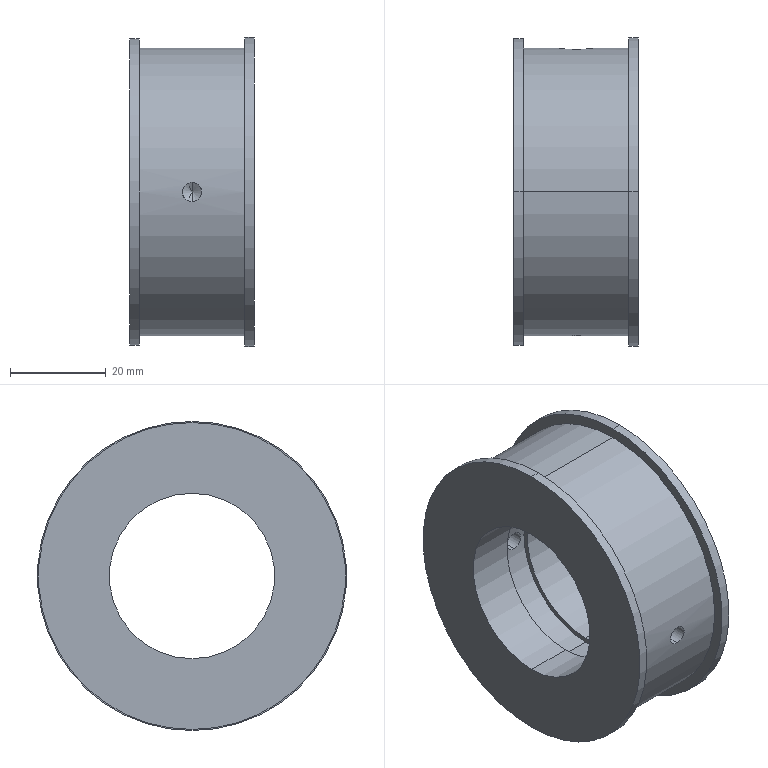Part | SolidWorks | features HoleWzd 3, Fillet 2, Revolution 1 | 1 solid | 31 faces | box 26 x 64.446 x 64.446 mm | volume 49939 mm3 | cylinder 18 | plane 7 | torus 2 | spline 2 | cone 2 | commonest cylinder face diameters 4 x4 34.5 x4 7.5 x2 36.5 x2 60 x2 64 x2
STEP:
#1=CARTESIAN_POINT('',(4.61,28.8,3.75));
#2=VERTEX_POINT('',#1);
#3=CARTESIAN_POINT('',(4.61,28.8,-3.75));
#4=VERTEX_POINT('',#3);
#5=CARTESIAN_POINT('',(4.61,28.8,0.));
#6=DIRECTION('',(0.,-1.,0.));
#7=DIRECTION('',(0.,0.,-1.));
#8=AXIS2_PLACEMENT_3D('',#5,#6,#7);
#9=CIRCLE('',#8,3.75);
#10=EDGE_CURVE('',#2,#4,#9,.T.);
#11=ORIENTED_EDGE('',*,*,#10,.F.);
#12=CARTESIAN_POINT('',(4.61,28.5,3.45));
#13=VERTEX_POINT('',#12);
#14=CARTESIAN_POINT('',(4.61,28.8,3.45));
#15=DIRECTION('',(1.,0.,0.));
#16=DIRECTION('',(0.,0.,-1.));
#17=AXIS2_PLACEMENT_3D('',#14,#15,#16);
#18=CIRCLE('',#17,0.3);
#19=EDGE_CURVE('',#2,#13,#18,.T.);
#20=ORIENTED_EDGE('',*,*,#19,.T.);
#21=CARTESIAN_POINT('',(4.61,28.5,-3.45));
#22=VERTEX_POINT('',#21);
#23=CARTESIAN_POINT('',(4.61,28.5,0.));
#24=DIRECTION('',(0.,1.,0.));
#25=DIRECTION('',(0.,0.,-1.));
#26=AXIS2_PLACEMENT_3D('',#23,#24,#25);
#27=CIRCLE('',#26,3.45);
#28=EDGE_CURVE('',#22,#13,#27,.T.);
#29=ORIENTED_EDGE('',*,*,#28,.F.);
#30=CARTESIAN_POINT('',(4.61,28.8,-3.45));
#31=DIRECTION('',(-1.,0.,0.));
#32=DIRECTION('',(0.,0.,1.));
#33=AXIS2_PLACEMENT_3D('',#30,#31,#32);
#34=CIRCLE('',#33,0.3);
#35=EDGE_CURVE('',#4,#22,#34,.T.);
#36=ORIENTED_EDGE('',*,*,#35,.F.);
#37=EDGE_LOOP('',(#11,#20,#29,#36));
#38=FACE_OUTER_BOUND('',#37,.T.);
#39=CARTESIAN_POINT('',(4.61,28.8,0.));
#40=DIRECTION('',(0.,-1.,0.));
#41=DIRECTION('',(0.,0.,-1.));
#42=AXIS2_PLACEMENT_3D('',#39,#40,#41);
#43=TOROIDAL_SURFACE('',#42,3.45,0.3);
#44=ADVANCED_FACE('',(#38),#43,.F.);
#45=CARTESIAN_POINT('',(3.758,29.551,-3.652));
#46=VERTEX_POINT('',#45);
#47=CARTESIAN_POINT('',(4.61,29.537,3.75));
#48=VERTEX_POINT('',#47);
#49=CARTESIAN_POINT('',(3.758,29.551,-3.652));
#50=CARTESIAN_POINT('',(3.535,29.558,-3.6));
#51=CARTESIAN_POINT('',(3.316,29.568,-3.527));
#52=CARTESIAN_POINT('',(2.899,29.591,-3.345));
#53=CARTESIAN_POINT('',(2.701,29.605,-3.236));
#54=CARTESIAN_POINT('',(2.325,29.634,-2.982));
#55=CARTESIAN_POINT('',(2.146,29.65,-2.836));
#56=CARTESIAN_POINT('',(1.822,29.682,-2.518));
#57=CARTESIAN_POINT('',(1.676,29.698,-2.346));
#58=CARTESIAN_POINT('',(1.414,29.728,-1.974));
#59=CARTESIAN_POINT('',(1.299,29.742,-1.774));
#60=CARTESIAN_POINT('',(1.109,29.766,-1.363));
#61=CARTESIAN_POINT('',(1.033,29.776,-1.149));
#62=CARTESIAN_POINT('',(0.9203,29.792,-0.7059));
#63=CARTESIAN_POINT('',(0.8842,29.797,-0.479));
#64=CARTESIAN_POINT('',(0.8536,29.801,-0.02683));
#65=CARTESIAN_POINT('',(0.8587,29.8,0.2003));
#66=CARTESIAN_POINT('',(0.9112,29.793,0.6567));
#67=CARTESIAN_POINT('',(0.9579,29.786,0.8794));
#68=CARTESIAN_POINT('',(1.09,29.769,1.312));
#69=CARTESIAN_POINT('',(1.177,29.757,1.524));
#70=CARTESIAN_POINT('',(1.387,29.731,1.93));
#71=CARTESIAN_POINT('',(1.509,29.717,2.121));
#72=CARTESIAN_POINT('',(1.787,29.686,2.478));
#73=CARTESIAN_POINT('',(1.944,29.67,2.647));
#74=CARTESIAN_POINT('',(2.284,29.638,2.95));
#75=CARTESIAN_POINT('',(2.466,29.623,3.084));
#76=CARTESIAN_POINT('',(2.853,29.594,3.32));
#77=CARTESIAN_POINT('',(3.06,29.581,3.422));
#78=CARTESIAN_POINT('',(3.485,29.56,3.584));
#79=CARTESIAN_POINT('',(3.703,29.552,3.646));
#80=CARTESIAN_POINT('',(4.15,29.54,3.729));
#81=CARTESIAN_POINT('',(4.38,29.537,3.75));
#82=CARTESIAN_POINT('',(4.61,29.537,3.75));
#83=B_SPLINE_CURVE_WITH_KNOTS('',3,(#49,#50,#51,#52,#53,#54,#55,#56,#57,#58,#59,#60,#61,#62,#63,#64,#65,#66,#67,#68,#69,#70,#71,#72,#73,#74,#75,#76,#77,#78,#79,#80,#81,#82),.UNSPECIFIED.,.F.,.F.,(4,2,2,2,2,2,2,2,2,2,2,2,2,2,2,2,4),(0.01269,0.01337,0.01406,0.01474,0.01543,0.01611,0.0168,0.01748,0.01817,0.01885,0.01954,0.02022,0.02091,0.02159,0.02228,0.02296,0.02365),.UNSPECIFIED.);
#84=EDGE_CURVE('',#46,#48,#83,.T.);
#85=ORIENTED_EDGE('',*,*,#84,.F.);
#86=CARTESIAN_POINT('',(3.712,29.749,-3.872));
#87=VERTEX_POINT('',#86);
#88=CARTESIAN_POINT('',(3.712,29.551,-3.847));
#89=DIRECTION('',(-0.9734,0.02959,0.2273));
#90=DIRECTION('',(0.2274,0.,0.9738));
#91=AXIS2_PLACEMENT_3D('',#88,#89,#90);
#92=CIRCLE('',#91,0.2);
#93=EDGE_CURVE('',#46,#87,#92,.T.);
#94=ORIENTED_EDGE('',*,*,#93,.T.);
#95=CARTESIAN_POINT('',(5.509,29.749,3.872));
#96=VERTEX_POINT('',#95);
#97=CARTESIAN_POINT('',(5.509,29.749,3.872));
#98=CARTESIAN_POINT('',(5.254,29.741,3.932));
#99=CARTESIAN_POINT('',(4.996,29.737,3.966));
#100=CARTESIAN_POINT('',(4.474,29.734,3.983));
#101=CARTESIAN_POINT('',(4.21,29.737,3.965));
#102=CARTESIAN_POINT('',(3.698,29.748,3.878));
#103=CARTESIAN_POINT('',(3.449,29.757,3.81));
#104=CARTESIAN_POINT('',(2.965,29.78,3.624));
#105=CARTESIAN_POINT('',(2.729,29.795,3.506));
#106=CARTESIAN_POINT('',(2.293,29.826,3.231));
#107=CARTESIAN_POINT('',(2.089,29.843,3.072));
#108=CARTESIAN_POINT('',(1.711,29.878,2.714));
#109=CARTESIAN_POINT('',(1.541,29.895,2.517));
#110=CARTESIAN_POINT('',(1.244,29.927,2.096));
#111=CARTESIAN_POINT('',(1.114,29.943,1.869));
#112=CARTESIAN_POINT('',(0.9018,29.969,1.394));
#113=CARTESIAN_POINT('',(0.82,29.979,1.149));
#114=CARTESIAN_POINT('',(0.7041,29.994,0.6447));
#115=CARTESIAN_POINT('',(0.6703,29.999,0.3829));
#116=CARTESIAN_POINT('',(0.6542,30.001,-0.135));
#117=CARTESIAN_POINT('',(0.6712,29.999,-0.3927));
#118=CARTESIAN_POINT('',(0.7555,29.987,-0.9056));
#119=CARTESIAN_POINT('',(0.8233,29.979,-1.16));
#120=CARTESIAN_POINT('',(1.004,29.956,-1.643));
#121=CARTESIAN_POINT('',(1.118,29.942,-1.876));
#122=CARTESIAN_POINT('',(1.392,29.911,-2.321));
#123=CARTESIAN_POINT('',(1.549,29.894,-2.526));
#124=CARTESIAN_POINT('',(1.9,29.86,-2.904));
#125=CARTESIAN_POINT('',(2.096,29.842,-3.078));
#126=CARTESIAN_POINT('',(2.516,29.809,-3.382));
#127=CARTESIAN_POINT('',(2.739,29.794,-3.512));
#128=CARTESIAN_POINT('',(3.21,29.768,-3.727));
#129=CARTESIAN_POINT('',(3.459,29.757,-3.813));
#130=CARTESIAN_POINT('',(3.712,29.749,-3.872));
#131=B_SPLINE_CURVE_WITH_KNOTS('',3,(#97,#98,#99,#100,#101,#102,#103,#104,#105,#106,#107,#108,#109,#110,#111,#112,#113,#114,#115,#116,#117,#118,#119,#120,#121,#122,#123,#124,#125,#126,#127,#128,#129,#130),.UNSPECIFIED.,.F.,.F.,(4,2,2,2,2,2,2,2,2,2,2,2,2,2,2,2,4),(0.02421,0.025,0.02578,0.02657,0.02735,0.02814,0.02892,0.02971,0.03049,0.03128,0.03206,0.03285,0.03363,0.03442,0.0352,0.03599,0.03677),.UNSPECIFIED.);
#132=EDGE_CURVE('',#96,#87,#131,.T.);
#133=ORIENTED_EDGE('',*,*,#132,.F.);
#134=CARTESIAN_POINT('',(5.463,29.551,3.652));
#135=VERTEX_POINT('',#134);
#136=CARTESIAN_POINT('',(5.509,29.551,3.846));
#137=DIRECTION('',(0.9734,0.02959,-0.2273));
#138=DIRECTION('',(-0.2274,0.,-0.9738));
#139=AXIS2_PLACEMENT_3D('',#136,#137,#138);
#140=CIRCLE('',#139,0.2);
#141=EDGE_CURVE('',#135,#96,#140,.T.);
#142=ORIENTED_EDGE('',*,*,#141,.F.);
#143=CARTESIAN_POINT('',(4.61,29.537,3.75));
#144=CARTESIAN_POINT('',(4.754,29.537,3.75));
#145=CARTESIAN_POINT('',(5.041,29.539,3.733));
#146=CARTESIAN_POINT('',(5.323,29.546,3.684));
#147=CARTESIAN_POINT('',(5.463,29.551,3.652));
#148=B_SPLINE_CURVE_WITH_KNOTS('',3,(#143,#144,#145,#146,#147),.UNSPECIFIED.,.F.,.F.,(4,1,4),(0.,0.0004293,0.0008586),.UNSPECIFIED.);
#149=EDGE_CURVE('',#48,#135,#148,.T.);
#150=ORIENTED_EDGE('',*,*,#149,.F.);
#151=EDGE_LOOP('',(#85,#94,#133,#142,#150));
#152=FACE_OUTER_BOUND('',#151,.T.);
#153=CARTESIAN_POINT('',(5.463,29.551,3.652));
#154=CARTESIAN_POINT('',(5.457,29.778,3.653));
#155=CARTESIAN_POINT('',(5.509,29.749,3.872));
#156=CARTESIAN_POINT('',(5.222,29.543,3.708));
#157=CARTESIAN_POINT('',(5.216,29.771,3.709));
#158=CARTESIAN_POINT('',(5.254,29.741,3.932));
#159=CARTESIAN_POINT('',(4.979,29.538,3.74));
#160=CARTESIAN_POINT('',(4.976,29.767,3.74));
#161=CARTESIAN_POINT('',(4.998,29.737,3.966));
#162=CARTESIAN_POINT('',(4.49,29.536,3.756));
#163=CARTESIAN_POINT('',(4.491,29.765,3.756));
#164=CARTESIAN_POINT('',(4.484,29.734,3.983));
#165=CARTESIAN_POINT('',(4.241,29.539,3.74));
#166=CARTESIAN_POINT('',(4.245,29.767,3.74));
#167=CARTESIAN_POINT('',(4.222,29.737,3.966));
#168=CARTESIAN_POINT('',(3.756,29.55,3.66));
#169=CARTESIAN_POINT('',(3.763,29.777,3.661));
#170=CARTESIAN_POINT('',(3.71,29.748,3.881));
#171=CARTESIAN_POINT('',(3.52,29.558,3.596));
#172=CARTESIAN_POINT('',(3.529,29.784,3.599));
#173=CARTESIAN_POINT('',(3.462,29.757,3.814));
#174=CARTESIAN_POINT('',(3.061,29.581,3.424));
#175=CARTESIAN_POINT('',(3.072,29.804,3.429));
#176=CARTESIAN_POINT('',(2.978,29.78,3.631));
#177=CARTESIAN_POINT('',(2.837,29.595,3.313));
#178=CARTESIAN_POINT('',(2.849,29.817,3.32));
#179=CARTESIAN_POINT('',(2.743,29.794,3.513));
#180=CARTESIAN_POINT('',(2.422,29.626,3.055));
#181=CARTESIAN_POINT('',(2.434,29.844,3.064));
#182=CARTESIAN_POINT('',(2.305,29.825,3.24));
#183=CARTESIAN_POINT('',(2.228,29.643,2.907));
#184=CARTESIAN_POINT('',(2.24,29.859,2.916));
#185=CARTESIAN_POINT('',(2.101,29.842,3.082));
#186=CARTESIAN_POINT('',(1.868,29.677,2.57));
#187=CARTESIAN_POINT('',(1.879,29.89,2.581));
#188=CARTESIAN_POINT('',(1.722,29.877,2.725));
#189=CARTESIAN_POINT('',(1.706,29.695,2.384));
#190=CARTESIAN_POINT('',(1.715,29.905,2.396));
#191=CARTESIAN_POINT('',(1.551,29.894,2.528));
#192=CARTESIAN_POINT('',(1.421,29.727,1.988));
#193=CARTESIAN_POINT('',(1.428,29.934,1.999));
#194=CARTESIAN_POINT('',(1.251,29.927,2.108));
#195=CARTESIAN_POINT('',(1.297,29.742,1.774));
#196=CARTESIAN_POINT('',(1.303,29.948,1.785));
#197=CARTESIAN_POINT('',(1.12,29.942,1.881));
#198=CARTESIAN_POINT('',(1.093,29.768,1.325));
#199=CARTESIAN_POINT('',(1.097,29.971,1.334));
#200=CARTESIAN_POINT('',(0.9058,29.968,1.405));
#201=CARTESIAN_POINT('',(1.015,29.779,1.093));
#202=CARTESIAN_POINT('',(1.017,29.981,1.101));
#203=CARTESIAN_POINT('',(0.8231,29.979,1.159));
#204=CARTESIAN_POINT('',(0.9033,29.794,0.6165));
#205=CARTESIAN_POINT('',(0.904,29.995,0.6213));
#206=CARTESIAN_POINT('',(0.7056,29.994,0.6537));
#207=CARTESIAN_POINT('',(0.8705,29.799,0.3687));
#208=CARTESIAN_POINT('',(0.8706,29.999,0.3714));
#209=CARTESIAN_POINT('',(0.671,29.999,0.391));
#210=CARTESIAN_POINT('',(0.8543,29.801,-0.1217));
#211=CARTESIAN_POINT('',(0.8542,30.001,-0.1225));
#212=CARTESIAN_POINT('',(0.654,30.001,-0.129));
#213=CARTESIAN_POINT('',(0.8701,29.799,-0.3657));
#214=CARTESIAN_POINT('',(0.8703,29.999,-0.3686));
#215=CARTESIAN_POINT('',(0.6706,29.999,-0.3878));
#216=CARTESIAN_POINT('',(0.95,29.788,-0.8512));
#217=CARTESIAN_POINT('',(0.9512,29.989,-0.8574));
#218=CARTESIAN_POINT('',(0.7547,29.988,-0.9027));
#219=CARTESIAN_POINT('',(1.014,29.779,-1.092));
#220=CARTESIAN_POINT('',(1.017,29.981,-1.1));
#221=CARTESIAN_POINT('',(0.8227,29.979,-1.158));
#222=CARTESIAN_POINT('',(1.187,29.756,-1.549));
#223=CARTESIAN_POINT('',(1.191,29.96,-1.559));
#224=CARTESIAN_POINT('',(1.004,29.956,-1.643));
#225=CARTESIAN_POINT('',(1.295,29.743,-1.769));
#226=CARTESIAN_POINT('',(1.301,29.948,-1.78));
#227=CARTESIAN_POINT('',(1.118,29.942,-1.876));
#228=CARTESIAN_POINT('',(1.556,29.711,-2.189));
#229=CARTESIAN_POINT('',(1.564,29.92,-2.201));
#230=CARTESIAN_POINT('',(1.393,29.911,-2.322));
#231=CARTESIAN_POINT('',(1.705,29.695,-2.383));
#232=CARTESIAN_POINT('',(1.714,29.905,-2.395));
#233=CARTESIAN_POINT('',(1.55,29.894,-2.527));
#234=CARTESIAN_POINT('',(2.038,29.661,-2.74));
#235=CARTESIAN_POINT('',(2.05,29.875,-2.751));
#236=CARTESIAN_POINT('',(1.901,29.86,-2.905));
#237=CARTESIAN_POINT('',(2.225,29.643,-2.904));
#238=CARTESIAN_POINT('',(2.237,29.859,-2.914));
#239=CARTESIAN_POINT('',(2.098,29.842,-3.08));
#240=CARTESIAN_POINT('',(2.624,29.61,-3.19));
#241=CARTESIAN_POINT('',(2.636,29.83,-3.198));
#242=CARTESIAN_POINT('',(2.518,29.809,-3.383));
#243=CARTESIAN_POINT('',(2.835,29.595,-3.312));
#244=CARTESIAN_POINT('',(2.847,29.817,-3.319));
#245=CARTESIAN_POINT('',(2.741,29.794,-3.512));
#246=CARTESIAN_POINT('',(3.282,29.569,-3.515));
#247=CARTESIAN_POINT('',(3.292,29.794,-3.519));
#248=CARTESIAN_POINT('',(3.211,29.768,-3.728));
#249=CARTESIAN_POINT('',(3.518,29.558,-3.596));
#250=CARTESIAN_POINT('',(3.527,29.784,-3.598));
#251=CARTESIAN_POINT('',(3.46,29.757,-3.813));
#252=CARTESIAN_POINT('',(3.758,29.551,-3.652));
#253=CARTESIAN_POINT('',(3.764,29.778,-3.653));
#254=CARTESIAN_POINT('',(3.712,29.749,-3.872));
#255=(BOUNDED_SURFACE()B_SPLINE_SURFACE(3,2,((#153,#154,#155),(#156,#157,#158),(#159,#160,#161),(#162,#163,#164),(#165,#166,#167),(#168,#169,#170),(#171,#172,#173),(#174,#175,#176),(#177,#178,#179),(#180,#181,#182),(#183,#184,#185),(#186,#187,#188),(#189,#190,#191),(#192,#193,#194),(#195,#196,#197),(#198,#199,#200),(#201,#202,#203),(#204,#205,#206),(#207,#208,#209),(#210,#211,#212),(#213,#214,#215),(#216,#217,#218),(#219,#220,#221),(#222,#223,#224),(#225,#226,#227),(#228,#229,#230),(#231,#232,#233),(#234,#235,#236),(#237,#238,#239),(#240,#241,#242),(#243,#244,#245),(#246,#247,#248),(#249,#250,#251),(#252,#253,#254)),.UNSPECIFIED.,.F.,.F.,.T.)B_SPLINE_SURFACE_WITH_KNOTS((4,2,2,2,2,2,2,2,2,2,2,2,2,2,2,2,4),(3,3),(0.,0.0007725,0.001545,0.002318,0.00309,0.003863,0.004635,0.005408,0.00618,0.006953,0.007725,0.008498,0.00927,0.01004,0.01082,0.01159,0.01236),(0.,1.),.UNSPECIFIED.)GEOMETRIC_REPRESENTATION_ITEM()RATIONAL_B_SPLINE_SURFACE(((1.,0.6612,1.),(1.,0.6597,1.),(1.,0.6588,1.),(1.,0.6584,1.),(1.,0.6589,1.),(1.,0.661,1.),(1.,0.6626,1.),(1.,0.6669,1.),(1.,0.6696,1.),(1.,0.6754,1.),(1.,0.6785,1.),(1.,0.6849,1.),(1.,0.688,1.),(1.,0.694,1.),(1.,0.6967,1.),(1.,0.7014,1.),(1.,0.7033,1.),(1.,0.706,1.),(1.,0.7069,1.),(1.,0.7073,1.),(1.,0.7069,1.),(1.,0.7049,1.),(1.,0.7033,1.),(1.,0.6992,1.),(1.,0.6968,1.),(1.,0.6911,1.),(1.,0.688,1.),(1.,0.6817,1.),(1.,0.6785,1.),(1.,0.6724,1.),(1.,0.6696,1.),(1.,0.6647,1.),(1.,0.6626,1.),(1.,0.6612,1.)))REPRESENTATION_ITEM('')SURFACE());
#256=ADVANCED_FACE('',(#152),#255,.T.);
#257=CARTESIAN_POINT('',(4.61,-24.798,0.));
#258=VERTEX_POINT('',#257);
#259=CARTESIAN_POINT('',(4.61,-26.,-2.));
#260=VERTEX_POINT('',#259);
#261=CARTESIAN_POINT('',(4.61,-26.,-2.));
#262=DIRECTION('',(0.,-0.515,-0.8572));
#263=VECTOR('',#262,1000.);
#264=LINE('',#261,#263);
#265=EDGE_CURVE('',#258,#260,#264,.T.);
#266=ORIENTED_EDGE('',*,*,#265,.F.);
#267=CARTESIAN_POINT('',(4.61,-26.,2.));
#268=VERTEX_POINT('',#267);
#269=CARTESIAN_POINT('',(4.61,-26.,2.));
#270=DIRECTION('',(0.,-0.515,0.8572));
#271=VECTOR('',#270,1000.);
#272=LINE('',#269,#271);
#273=EDGE_CURVE('',#258,#268,#272,.T.);
#274=ORIENTED_EDGE('',*,*,#273,.T.);
#275=CARTESIAN_POINT('',(4.61,-26.,0.));
#276=DIRECTION('',(0.,-1.,0.));
#277=DIRECTION('',(0.,0.,-1.));
#278=AXIS2_PLACEMENT_3D('',#275,#276,#277);
#279=CIRCLE('',#278,2.);
#280=EDGE_CURVE('',#268,#260,#279,.T.);
#281=ORIENTED_EDGE('',*,*,#280,.T.);
#282=EDGE_LOOP('',(#266,#274,#281));
#283=FACE_OUTER_BOUND('',#282,.T.);
#284=CARTESIAN_POINT('',(4.61,-26.,0.));
#285=DIRECTION('',(0.,-1.,0.));
#286=DIRECTION('',(0.,0.,-1.));
#287=AXIS2_PLACEMENT_3D('',#284,#285,#286);
#288=CONICAL_SURFACE('',#287,2.,1.03);
#289=ADVANCED_FACE('',(#283),#288,.F.);
#290=ORIENTED_EDGE('',*,*,#280,.F.);
#291=CARTESIAN_POINT('',(4.61,-29.933,2.));
#292=VERTEX_POINT('',#291);
#293=CARTESIAN_POINT('',(4.61,-30.,2.));
#294=DIRECTION('',(0.,-1.,0.));
#295=VECTOR('',#294,1000.);
#296=LINE('',#293,#295);
#297=EDGE_CURVE('',#268,#292,#296,.T.);
#298=ORIENTED_EDGE('',*,*,#297,.T.);
#299=CARTESIAN_POINT('',(4.61,-29.933,-2.));
#300=VERTEX_POINT('',#299);
#301=CARTESIAN_POINT('',(4.61,-29.933,-2.));
#302=CARTESIAN_POINT('',(4.478,-29.933,-2.));
#303=CARTESIAN_POINT('',(4.348,-29.934,-1.987));
#304=CARTESIAN_POINT('',(4.093,-29.937,-1.936));
#305=CARTESIAN_POINT('',(3.965,-29.94,-1.898));
#306=CARTESIAN_POINT('',(3.723,-29.946,-1.797));
#307=CARTESIAN_POINT('',(3.608,-29.95,-1.736));
#308=CARTESIAN_POINT('',(3.391,-29.958,-1.591));
#309=CARTESIAN_POINT('',(3.288,-29.962,-1.506));
#310=CARTESIAN_POINT('',(3.011,-29.975,-1.229));
#311=CARTESIAN_POINT('',(2.862,-29.984,-1.006));
#312=CARTESIAN_POINT('',(2.663,-29.996,-0.525));
#313=CARTESIAN_POINT('',(2.61,-30.,-0.2617));
#314=CARTESIAN_POINT('',(2.61,-30.,0.1298));
#315=CARTESIAN_POINT('',(2.623,-29.999,0.2623));
#316=CARTESIAN_POINT('',(2.674,-29.996,0.5189));
#317=CARTESIAN_POINT('',(2.712,-29.993,0.6436));
#318=CARTESIAN_POINT('',(2.812,-29.987,0.8858));
#319=CARTESIAN_POINT('',(2.875,-29.983,1.003));
#320=CARTESIAN_POINT('',(3.02,-29.975,1.22));
#321=CARTESIAN_POINT('',(3.102,-29.971,1.321));
#322=CARTESIAN_POINT('',(3.289,-29.962,1.507));
#323=CARTESIAN_POINT('',(3.39,-29.958,1.59));
#324=CARTESIAN_POINT('',(3.607,-29.95,1.735));
#325=CARTESIAN_POINT('',(3.724,-29.946,1.798));
#326=CARTESIAN_POINT('',(3.966,-29.94,1.898));
#327=CARTESIAN_POINT('',(4.091,-29.937,1.936));
#328=CARTESIAN_POINT('',(4.347,-29.934,1.987));
#329=CARTESIAN_POINT('',(4.48,-29.933,2.));
#330=CARTESIAN_POINT('',(4.61,-29.933,2.));
#331=B_SPLINE_CURVE_WITH_KNOTS('',3,(#301,#302,#303,#304,#305,#306,#307,#308,#309,#310,#311,#312,#313,#314,#315,#316,#317,#318,#319,#320,#321,#322,#323,#324,#325,#326,#327,#328,#329,#330),.UNSPECIFIED.,.F.,.F.,(4,2,2,2,2,2,2,2,2,2,2,2,2,2,4),(0.,0.0003909,0.0007818,0.001173,0.001564,0.002345,0.003127,0.003518,0.003909,0.0043,0.004691,0.005082,0.005473,0.005864,0.006255),.UNSPECIFIED.);
#332=EDGE_CURVE('',#300,#292,#331,.T.);
#333=ORIENTED_EDGE('',*,*,#332,.F.);
#334=CARTESIAN_POINT('',(4.61,-30.,-2.));
#335=DIRECTION('',(0.,-1.,0.));
#336=VECTOR('',#335,1000.);
#337=LINE('',#334,#336);
#338=EDGE_CURVE('',#260,#300,#337,.T.);
#339=ORIENTED_EDGE('',*,*,#338,.F.);
#340=EDGE_LOOP('',(#290,#298,#333,#339));
#341=FACE_OUTER_BOUND('',#340,.T.);
#342=CARTESIAN_POINT('',(4.61,-30.,0.));
#343=DIRECTION('',(0.,-1.,0.));
#344=DIRECTION('',(0.,0.,-1.));
#345=AXIS2_PLACEMENT_3D('',#342,#343,#344);
#346=CYLINDRICAL_SURFACE('',#345,2.);
#347=ADVANCED_FACE('',(#341),#346,.F.);
#348=CARTESIAN_POINT('',(4.61,18.14,-2.));
#349=VERTEX_POINT('',#348);
#350=CARTESIAN_POINT('',(4.61,18.14,2.));
#351=VERTEX_POINT('',#350);
#352=CARTESIAN_POINT('',(4.61,18.14,-2.));
#353=CARTESIAN_POINT('',(4.349,18.14,-2.));
#354=CARTESIAN_POINT('',(4.086,18.146,-1.948));
#355=CARTESIAN_POINT('',(3.605,18.166,-1.748));
#356=CARTESIAN_POINT('',(3.382,18.181,-1.599));
#357=CARTESIAN_POINT('',(3.105,18.202,-1.323));
#358=CARTESIAN_POINT('',(3.02,18.209,-1.22));
#359=CARTESIAN_POINT('',(2.875,18.223,-1.003));
#360=CARTESIAN_POINT('',(2.814,18.229,-0.8884));
#361=CARTESIAN_POINT('',(2.713,18.239,-0.6463));
#362=CARTESIAN_POINT('',(2.675,18.243,-0.5193));
#363=CARTESIAN_POINT('',(2.624,18.249,-0.2636));
#364=CARTESIAN_POINT('',(2.61,18.25,-0.1337));
#365=CARTESIAN_POINT('',(2.61,18.25,0.1307));
#366=CARTESIAN_POINT('',(2.623,18.249,0.2608));
#367=CARTESIAN_POINT('',(2.674,18.243,0.5165));
#368=CARTESIAN_POINT('',(2.712,18.239,0.6436));
#369=CARTESIAN_POINT('',(2.812,18.229,0.8858));
#370=CARTESIAN_POINT('',(2.874,18.223,1.001));
#371=CARTESIAN_POINT('',(3.019,18.21,1.218));
#372=CARTESIAN_POINT('',(3.103,18.202,1.321));
#373=CARTESIAN_POINT('',(3.379,18.181,1.598));
#374=CARTESIAN_POINT('',(3.602,18.166,1.747));
#375=CARTESIAN_POINT('',(4.083,18.146,1.947));
#376=CARTESIAN_POINT('',(4.346,18.14,2.));
#377=CARTESIAN_POINT('',(4.61,18.14,2.));
#378=B_SPLINE_CURVE_WITH_KNOTS('',3,(#352,#353,#354,#355,#356,#357,#358,#359,#360,#361,#362,#363,#364,#365,#366,#367,#368,#369,#370,#371,#372,#373,#374,#375,#376,#377),.UNSPECIFIED.,.F.,.F.,(4,2,2,2,2,2,2,2,2,2,2,2,4),(0.006258,0.00704,0.007822,0.008213,0.008604,0.008995,0.009386,0.009777,0.01017,0.01056,0.01095,0.01173,0.01251),.UNSPECIFIED.);
#379=EDGE_CURVE('',#349,#351,#378,.T.);
#380=ORIENTED_EDGE('',*,*,#379,.F.);
#381=CARTESIAN_POINT('',(4.61,28.5,-2.));
#382=VERTEX_POINT('',#381);
#383=CARTESIAN_POINT('',(4.61,28.5,-2.));
#384=DIRECTION('',(0.,1.,0.));
#385=VECTOR('',#384,1000.);
#386=LINE('',#383,#385);
#387=EDGE_CURVE('',#349,#382,#386,.T.);
#388=ORIENTED_EDGE('',*,*,#387,.T.);
#389=CARTESIAN_POINT('',(4.61,28.5,2.));
#390=VERTEX_POINT('',#389);
#391=CARTESIAN_POINT('',(4.61,28.5,0.));
#392=DIRECTION('',(0.,1.,0.));
#393=DIRECTION('',(0.,0.,1.));
#394=AXIS2_PLACEMENT_3D('',#391,#392,#393);
#395=CIRCLE('',#394,2.);
#396=EDGE_CURVE('',#382,#390,#395,.T.);
#397=ORIENTED_EDGE('',*,*,#396,.T.);
#398=CARTESIAN_POINT('',(4.61,28.5,2.));
#399=DIRECTION('',(0.,1.,0.));
#400=VECTOR('',#399,1000.);
#401=LINE('',#398,#400);
#402=EDGE_CURVE('',#351,#390,#401,.T.);
#403=ORIENTED_EDGE('',*,*,#402,.F.);
#404=EDGE_LOOP('',(#380,#388,#397,#403));
#405=FACE_OUTER_BOUND('',#404,.T.);
#406=CARTESIAN_POINT('',(4.61,28.5,0.));
#407=DIRECTION('',(0.,1.,0.));
#408=DIRECTION('',(0.,0.,1.));
#409=AXIS2_PLACEMENT_3D('',#406,#407,#408);
#410=CYLINDRICAL_SURFACE('',#409,2.);
#411=ADVANCED_FACE('',(#405),#410,.F.);
#412=ORIENTED_EDGE('',*,*,#10,.T.);
#413=CARTESIAN_POINT('',(4.61,29.537,-3.75));
#414=VERTEX_POINT('',#413);
#415=CARTESIAN_POINT('',(4.61,30.,-3.75));
#416=DIRECTION('',(0.,1.,0.));
#417=VECTOR('',#416,1000.);
#418=LINE('',#415,#417);
#419=EDGE_CURVE('',#4,#414,#418,.T.);
#420=ORIENTED_EDGE('',*,*,#419,.T.);
#421=CARTESIAN_POINT('',(4.61,29.537,-3.75));
#422=CARTESIAN_POINT('',(4.468,29.537,-3.75));
#423=CARTESIAN_POINT('',(4.325,29.538,-3.742));
#424=CARTESIAN_POINT('',(4.038,29.543,-3.709));
#425=CARTESIAN_POINT('',(3.897,29.546,-3.684));
#426=CARTESIAN_POINT('',(3.758,29.551,-3.652));
#427=B_SPLINE_CURVE_WITH_KNOTS('',3,(#421,#422,#423,#424,#425,#426),.UNSPECIFIED.,.F.,.F.,(4,2,4),(0.01183,0.01226,0.01269),.UNSPECIFIED.);
#428=EDGE_CURVE('',#414,#46,#427,.T.);
#429=ORIENTED_EDGE('',*,*,#428,.T.);
#430=ORIENTED_EDGE('',*,*,#84,.T.);
#431=CARTESIAN_POINT('',(4.61,30.,3.75));
#432=DIRECTION('',(0.,1.,0.));
#433=VECTOR('',#432,1000.);
#434=LINE('',#431,#433);
#435=EDGE_CURVE('',#2,#48,#434,.T.);
#436=ORIENTED_EDGE('',*,*,#435,.F.);
#437=EDGE_LOOP('',(#412,#420,#429,#430,#436));
#438=FACE_OUTER_BOUND('',#437,.T.);
#439=CARTESIAN_POINT('',(4.61,30.,0.));
#440=DIRECTION('',(0.,1.,0.));
#441=DIRECTION('',(0.,0.,1.));
#442=AXIS2_PLACEMENT_3D('',#439,#440,#441);
#443=CYLINDRICAL_SURFACE('',#442,3.75);
#444=ADVANCED_FACE('',(#438),#443,.F.);
#445=CARTESIAN_POINT('',(1.61,0.,-17.25));
#446=VERTEX_POINT('',#445);
#447=CARTESIAN_POINT('',(1.61,0.,17.25));
#448=VERTEX_POINT('',#447);
#449=CARTESIAN_POINT('',(1.61,0.,0.));
#450=DIRECTION('',(-1.,0.,0.));
#451=DIRECTION('',(0.,0.,1.));
#452=AXIS2_PLACEMENT_3D('',#449,#450,#451);
#453=CIRCLE('',#452,17.25);
#454=EDGE_CURVE('',#446,#448,#453,.T.);
#455=ORIENTED_EDGE('',*,*,#454,.F.);
#456=CARTESIAN_POINT('',(-8.39,0.,-17.25));
#457=VERTEX_POINT('',#456);
#458=CARTESIAN_POINT('',(-19.037,0.,-17.25));
#459=DIRECTION('',(-1.,0.,0.));
#460=VECTOR('',#459,1000.);
#461=LINE('',#458,#460);
#462=EDGE_CURVE('',#446,#457,#461,.T.);
#463=ORIENTED_EDGE('',*,*,#462,.T.);
#464=CARTESIAN_POINT('',(-8.39,0.,17.25));
#465=VERTEX_POINT('',#464);
#466=CARTESIAN_POINT('',(-8.39,0.,0.));
#467=DIRECTION('',(-1.,0.,0.));
#468=DIRECTION('',(0.,0.,1.));
#469=AXIS2_PLACEMENT_3D('',#466,#467,#468);
#470=CIRCLE('',#469,17.25);
#471=EDGE_CURVE('',#457,#465,#470,.T.);
#472=ORIENTED_EDGE('',*,*,#471,.T.);
#473=CARTESIAN_POINT('',(-19.037,0.,17.25));
#474=DIRECTION('',(-1.,0.,0.));
#475=VECTOR('',#474,1000.);
#476=LINE('',#473,#475);
#477=EDGE_CURVE('',#448,#465,#476,.T.);
#478=ORIENTED_EDGE('',*,*,#477,.F.);
#479=EDGE_LOOP('',(#455,#463,#472,#478));
#480=FACE_OUTER_BOUND('',#479,.T.);
#481=CARTESIAN_POINT('',(-19.037,0.,0.));
#482=DIRECTION('',(-1.,0.,0.));
#483=DIRECTION('',(0.,0.,1.));
#484=AXIS2_PLACEMENT_3D('',#481,#482,#483);
#485=CYLINDRICAL_SURFACE('',#484,17.25);
#486=ADVANCED_FACE('',(#480),#485,.F.);
#487=CARTESIAN_POINT('',(7.61,0.,-18.25));
#488=VERTEX_POINT('',#487);
#489=CARTESIAN_POINT('',(7.61,0.,18.25));
#490=VERTEX_POINT('',#489);
#491=CARTESIAN_POINT('',(7.61,0.,0.));
#492=DIRECTION('',(-1.,0.,0.));
#493=DIRECTION('',(0.,0.,1.));
#494=AXIS2_PLACEMENT_3D('',#491,#492,#493);
#495=CIRCLE('',#494,18.25);
#496=EDGE_CURVE('',#488,#490,#495,.T.);
#497=ORIENTED_EDGE('',*,*,#496,.F.);
#498=CARTESIAN_POINT('',(1.61,0.,-18.25));
#499=VERTEX_POINT('',#498);
#500=CARTESIAN_POINT('',(-19.037,0.,-18.25));
#501=DIRECTION('',(-1.,0.,0.));
#502=VECTOR('',#501,1000.);
#503=LINE('',#500,#502);
#504=EDGE_CURVE('',#488,#499,#503,.T.);
#505=ORIENTED_EDGE('',*,*,#504,.T.);
#506=CARTESIAN_POINT('',(1.61,0.,18.25));
#507=VERTEX_POINT('',#506);
#508=CARTESIAN_POINT('',(1.61,0.,0.));
#509=DIRECTION('',(-1.,0.,0.));
#510=DIRECTION('',(0.,0.,1.));
#511=AXIS2_PLACEMENT_3D('',#508,#509,#510);
#512=CIRCLE('',#511,18.25);
#513=EDGE_CURVE('',#499,#507,#512,.T.);
#514=ORIENTED_EDGE('',*,*,#513,.T.);
#515=CARTESIAN_POINT('',(-19.037,0.,18.25));
#516=DIRECTION('',(-1.,0.,0.));
#517=VECTOR('',#516,1000.);
#518=LINE('',#515,#517);
#519=EDGE_CURVE('',#490,#507,#518,.T.);
#520=ORIENTED_EDGE('',*,*,#519,.F.);
#521=EDGE_LOOP('',(#497,#505,#514,#520));
#522=FACE_OUTER_BOUND('',#521,.T.);
#523=CARTESIAN_POINT('',(-19.037,0.,0.));
#524=DIRECTION('',(-1.,0.,0.));
#525=DIRECTION('',(0.,0.,1.));
#526=AXIS2_PLACEMENT_3D('',#523,#524,#525);
#527=CYLINDRICAL_SURFACE('',#526,18.25);
#528=ADVANCED_FACE('',(#522),#527,.F.);
#529=CARTESIAN_POINT('',(17.61,0.,-17.25));
#530=VERTEX_POINT('',#529);
#531=CARTESIAN_POINT('',(17.61,0.,17.25));
#532=VERTEX_POINT('',#531);
#533=CARTESIAN_POINT('',(17.61,0.,0.));
#534=DIRECTION('',(-1.,0.,0.));
#535=DIRECTION('',(0.,0.,1.));
#536=AXIS2_PLACEMENT_3D('',#533,#534,#535);
#537=CIRCLE('',#536,17.25);
#538=EDGE_CURVE('',#530,#532,#537,.T.);
#539=ORIENTED_EDGE('',*,*,#538,.F.);
#540=CARTESIAN_POINT('',(7.61,0.,-17.25));
#541=VERTEX_POINT('',#540);
#542=CARTESIAN_POINT('',(-19.037,0.,-17.25));
#543=DIRECTION('',(-1.,0.,0.));
#544=VECTOR('',#543,1000.);
#545=LINE('',#542,#544);
#546=EDGE_CURVE('',#530,#541,#545,.T.);
#547=ORIENTED_EDGE('',*,*,#546,.T.);
#548=CARTESIAN_POINT('',(7.61,0.,17.25));
#549=VERTEX_POINT('',#548);
#550=CARTESIAN_POINT('',(7.61,0.,0.));
#551=DIRECTION('',(-1.,0.,0.));
#552=DIRECTION('',(0.,0.,1.));
#553=AXIS2_PLACEMENT_3D('',#550,#551,#552);
#554=CIRCLE('',#553,17.25);
#555=EDGE_CURVE('',#541,#549,#554,.T.);
#556=ORIENTED_EDGE('',*,*,#555,.T.);
#557=CARTESIAN_POINT('',(-19.037,0.,17.25));
#558=DIRECTION('',(-1.,0.,0.));
#559=VECTOR('',#558,1000.);
#560=LINE('',#557,#559);
#561=EDGE_CURVE('',#532,#549,#560,.T.);
#562=ORIENTED_EDGE('',*,*,#561,.F.);
#563=EDGE_LOOP('',(#539,#547,#556,#562));
#564=FACE_OUTER_BOUND('',#563,.T.);
#565=CARTESIAN_POINT('',(-19.037,0.,0.));
#566=DIRECTION('',(-1.,0.,0.));
#567=DIRECTION('',(0.,0.,1.));
#568=AXIS2_PLACEMENT_3D('',#565,#566,#567);
#569=CYLINDRICAL_SURFACE('',#568,17.25);
#570=ADVANCED_FACE('',(#564),#569,.F.);
#571=CARTESIAN_POINT('',(17.61,0.,32.223));
#572=VERTEX_POINT('',#571);
#573=CARTESIAN_POINT('',(17.61,0.,-32.223));
#574=VERTEX_POINT('',#573);
#575=CARTESIAN_POINT('',(17.61,0.,0.));
#576=DIRECTION('',(-1.,0.,0.));
#577=DIRECTION('',(0.,0.,1.));
#578=AXIS2_PLACEMENT_3D('',#575,#576,#577);
#579=CIRCLE('',#578,32.223);
#580=EDGE_CURVE('',#572,#574,#579,.T.);
#581=ORIENTED_EDGE('',*,*,#580,.T.);
#582=CARTESIAN_POINT('',(15.61,0.,-32.223));
#583=VERTEX_POINT('',#582);
#584=CARTESIAN_POINT('',(-19.037,0.,-32.223));
#585=DIRECTION('',(-1.,0.,0.));
#586=VECTOR('',#585,1000.);
#587=LINE('',#584,#586);
#588=EDGE_CURVE('',#574,#583,#587,.T.);
#589=ORIENTED_EDGE('',*,*,#588,.T.);
#590=CARTESIAN_POINT('',(15.61,0.,32.223));
#591=VERTEX_POINT('',#590);
#592=CARTESIAN_POINT('',(15.61,0.,0.));
#593=DIRECTION('',(-1.,0.,0.));
#594=DIRECTION('',(0.,0.,1.));
#595=AXIS2_PLACEMENT_3D('',#592,#593,#594);
#596=CIRCLE('',#595,32.223);
#597=EDGE_CURVE('',#591,#583,#596,.T.);
#598=ORIENTED_EDGE('',*,*,#597,.F.);
#599=CARTESIAN_POINT('',(-19.037,0.,32.223));
#600=DIRECTION('',(-1.,0.,0.));
#601=VECTOR('',#600,1000.);
#602=LINE('',#599,#601);
#603=EDGE_CURVE('',#572,#591,#602,.T.);
#604=ORIENTED_EDGE('',*,*,#603,.F.);
#605=EDGE_LOOP('',(#581,#589,#598,#604));
#606=FACE_OUTER_BOUND('',#605,.T.);
#607=CARTESIAN_POINT('',(-19.037,0.,0.));
#608=DIRECTION('',(-1.,0.,0.));
#609=DIRECTION('',(0.,0.,1.));
#610=AXIS2_PLACEMENT_3D('',#607,#608,#609);
#611=CYLINDRICAL_SURFACE('',#610,32.223);
#612=ADVANCED_FACE('',(#606),#611,.T.);
#613=ORIENTED_EDGE('',*,*,#132,.T.);
#614=CARTESIAN_POINT('',(3.712,29.749,-3.872));
#615=CARTESIAN_POINT('',(3.965,29.741,-3.932));
#616=CARTESIAN_POINT('',(4.227,29.737,-3.966));
#617=CARTESIAN_POINT('',(4.746,29.734,-3.983));
#618=CARTESIAN_POINT('',(5.003,29.737,-3.965));
#619=CARTESIAN_POINT('',(5.516,29.748,-3.879));
#620=CARTESIAN_POINT('',(5.77,29.757,-3.81));
#621=CARTESIAN_POINT('',(6.253,29.78,-3.626));
#622=CARTESIAN_POINT('',(6.484,29.794,-3.51));
#623=CARTESIAN_POINT('',(6.927,29.826,-3.232));
#624=CARTESIAN_POINT('',(7.131,29.843,-3.073));
#625=CARTESIAN_POINT('',(7.505,29.877,-2.718));
#626=CARTESIAN_POINT('',(7.677,29.895,-2.519));
#627=CARTESIAN_POINT('',(7.977,29.927,-2.096));
#628=CARTESIAN_POINT('',(8.105,29.942,-1.872));
#629=CARTESIAN_POINT('',(8.317,29.968,-1.399));
#630=CARTESIAN_POINT('',(8.401,29.979,-1.149));
#631=CARTESIAN_POINT('',(8.517,29.994,-0.6445));
#632=CARTESIAN_POINT('',(8.55,29.999,-0.3881));
#633=CARTESIAN_POINT('',(8.567,30.001,0.1335));
#634=CARTESIAN_POINT('',(8.549,29.998,0.3946));
#635=CARTESIAN_POINT('',(8.465,29.987,0.9045));
#636=CARTESIAN_POINT('',(8.398,29.979,1.157));
#637=CARTESIAN_POINT('',(8.216,29.956,1.646));
#638=CARTESIAN_POINT('',(8.102,29.942,1.877));
#639=CARTESIAN_POINT('',(7.831,29.911,2.317));
#640=CARTESIAN_POINT('',(7.671,29.894,2.527));
#641=CARTESIAN_POINT('',(7.319,29.86,2.906));
#642=CARTESIAN_POINT('',(7.126,29.842,3.077));
#643=CARTESIAN_POINT('',(6.705,29.809,3.381));
#644=CARTESIAN_POINT('',(6.478,29.794,3.514));
#645=CARTESIAN_POINT('',(6.008,29.768,3.728));
#646=CARTESIAN_POINT('',(5.764,29.757,3.812));
#647=CARTESIAN_POINT('',(5.509,29.749,3.872));
#648=B_SPLINE_CURVE_WITH_KNOTS('',3,(#614,#615,#616,#617,#618,#619,#620,#621,#622,#623,#624,#625,#626,#627,#628,#629,#630,#631,#632,#633,#634,#635,#636,#637,#638,#639,#640,#641,#642,#643,#644,#645,#646,#647),.UNSPECIFIED.,.F.,.F.,(4,2,2,2,2,2,2,2,2,2,2,2,2,2,2,2,4),(0.01165,0.01243,0.01322,0.014,0.01479,0.01557,0.01636,0.01714,0.01793,0.01872,0.0195,0.02029,0.02107,0.02186,0.02264,0.02343,0.02421),.UNSPECIFIED.);
#649=EDGE_CURVE('',#87,#96,#648,.T.);
#650=ORIENTED_EDGE('',*,*,#649,.T.);
#651=EDGE_LOOP('',(#613,#650));
#652=FACE_BOUND('',#651,.T.);
#653=CARTESIAN_POINT('',(15.61,0.,30.));
#654=VERTEX_POINT('',#653);
#655=CARTESIAN_POINT('',(15.61,0.,-30.));
#656=VERTEX_POINT('',#655);
#657=CARTESIAN_POINT('',(15.61,0.,0.));
#658=DIRECTION('',(-1.,0.,0.));
#659=DIRECTION('',(0.,0.,1.));
#660=AXIS2_PLACEMENT_3D('',#657,#658,#659);
#661=CIRCLE('',#660,30.);
#662=EDGE_CURVE('',#654,#656,#661,.T.);
#663=ORIENTED_EDGE('',*,*,#662,.T.);
#664=CARTESIAN_POINT('',(-6.39,0.,-30.));
#665=VERTEX_POINT('',#664);
#666=CARTESIAN_POINT('',(-19.037,0.,-30.));
#667=DIRECTION('',(-1.,0.,0.));
#668=VECTOR('',#667,1000.);
#669=LINE('',#666,#668);
#670=EDGE_CURVE('',#656,#665,#669,.T.);
#671=ORIENTED_EDGE('',*,*,#670,.T.);
#672=CARTESIAN_POINT('',(-6.39,0.,30.));
#673=VERTEX_POINT('',#672);
#674=CARTESIAN_POINT('',(-6.39,0.,0.));
#675=DIRECTION('',(-1.,0.,0.));
#676=DIRECTION('',(0.,0.,1.));
#677=AXIS2_PLACEMENT_3D('',#674,#675,#676);
#678=CIRCLE('',#677,30.);
#679=EDGE_CURVE('',#673,#665,#678,.T.);
#680=ORIENTED_EDGE('',*,*,#679,.F.);
#681=CARTESIAN_POINT('',(-19.037,0.,30.));
#682=DIRECTION('',(-1.,0.,0.));
#683=VECTOR('',#682,1000.);
#684=LINE('',#681,#683);
#685=EDGE_CURVE('',#654,#673,#684,.T.);
#686=ORIENTED_EDGE('',*,*,#685,.F.);
#687=EDGE_LOOP('',(#663,#671,#680,#686));
#688=FACE_OUTER_BOUND('',#687,.T.);
#689=CARTESIAN_POINT('',(-19.037,0.,0.));
#690=DIRECTION('',(-1.,0.,0.));
#691=DIRECTION('',(0.,0.,1.));
#692=AXIS2_PLACEMENT_3D('',#689,#690,#691);
#693=CYLINDRICAL_SURFACE('',#692,30.);
#694=ADVANCED_FACE('',(#652,#688),#693,.T.);
#695=CARTESIAN_POINT('',(-6.39,0.,32.));
#696=VERTEX_POINT('',#695);
#697=CARTESIAN_POINT('',(-6.39,0.,-32.));
#698=VERTEX_POINT('',#697);
#699=CARTESIAN_POINT('',(-6.39,0.,0.));
#700=DIRECTION('',(-1.,0.,0.));
#701=DIRECTION('',(0.,0.,1.));
#702=AXIS2_PLACEMENT_3D('',#699,#700,#701);
#703=CIRCLE('',#702,32.);
#704=EDGE_CURVE('',#696,#698,#703,.T.);
#705=ORIENTED_EDGE('',*,*,#704,.T.);
#706=CARTESIAN_POINT('',(-8.39,0.,-32.));
#707=VERTEX_POINT('',#706);
#708=CARTESIAN_POINT('',(-19.037,0.,-32.));
#709=DIRECTION('',(-1.,0.,0.));
#710=VECTOR('',#709,1000.);
#711=LINE('',#708,#710);
#712=EDGE_CURVE('',#698,#707,#711,.T.);
#713=ORIENTED_EDGE('',*,*,#712,.T.);
#714=CARTESIAN_POINT('',(-8.39,0.,32.));
#715=VERTEX_POINT('',#714);
#716=CARTESIAN_POINT('',(-8.39,0.,0.));
#717=DIRECTION('',(-1.,0.,0.));
#718=DIRECTION('',(0.,0.,1.));
#719=AXIS2_PLACEMENT_3D('',#716,#717,#718);
#720=CIRCLE('',#719,32.);
#721=EDGE_CURVE('',#715,#707,#720,.T.);
#722=ORIENTED_EDGE('',*,*,#721,.F.);
#723=CARTESIAN_POINT('',(-19.037,0.,32.));
#724=DIRECTION('',(-1.,0.,0.));
#725=VECTOR('',#724,1000.);
#726=LINE('',#723,#725);
#727=EDGE_CURVE('',#696,#715,#726,.T.);
#728=ORIENTED_EDGE('',*,*,#727,.F.);
#729=EDGE_LOOP('',(#705,#713,#722,#728));
#730=FACE_OUTER_BOUND('',#729,.T.);
#731=CARTESIAN_POINT('',(-19.037,0.,0.));
#732=DIRECTION('',(-1.,0.,0.));
#733=DIRECTION('',(0.,0.,1.));
#734=AXIS2_PLACEMENT_3D('',#731,#732,#733);
#735=CYLINDRICAL_SURFACE('',#734,32.);
#736=ADVANCED_FACE('',(#730),#735,.T.);
#737=ORIENTED_EDGE('',*,*,#712,.F.);
#738=CARTESIAN_POINT('',(-6.39,0.,0.));
#739=DIRECTION('',(-1.,0.,0.));
#740=DIRECTION('',(0.,0.,1.));
#741=AXIS2_PLACEMENT_3D('',#738,#739,#740);
#742=CIRCLE('',#741,32.);
#743=EDGE_CURVE('',#698,#696,#742,.T.);
#744=ORIENTED_EDGE('',*,*,#743,.T.);
#745=ORIENTED_EDGE('',*,*,#727,.T.);
#746=CARTESIAN_POINT('',(-8.39,0.,0.));
#747=DIRECTION('',(-1.,0.,0.));
#748=DIRECTION('',(0.,0.,1.));
#749=AXIS2_PLACEMENT_3D('',#746,#747,#748);
#750=CIRCLE('',#749,32.);
#751=EDGE_CURVE('',#707,#715,#750,.T.);
#752=ORIENTED_EDGE('',*,*,#751,.F.);
#753=EDGE_LOOP('',(#737,#744,#745,#752));
#754=FACE_OUTER_BOUND('',#753,.T.);
#755=CARTESIAN_POINT('',(-19.037,0.,0.));
#756=DIRECTION('',(-1.,0.,0.));
#757=DIRECTION('',(0.,0.,1.));
#758=AXIS2_PLACEMENT_3D('',#755,#756,#757);
#759=CYLINDRICAL_SURFACE('',#758,32.);
#760=ADVANCED_FACE('',(#754),#759,.T.);
#761=ORIENTED_EDGE('',*,*,#704,.F.);
#762=ORIENTED_EDGE('',*,*,#743,.F.);
#763=EDGE_LOOP('',(#761,#762));
#764=FACE_OUTER_BOUND('',#763,.T.);
#765=ORIENTED_EDGE('',*,*,#679,.T.);
#766=CARTESIAN_POINT('',(-6.39,0.,0.));
#767=DIRECTION('',(-1.,0.,0.));
#768=DIRECTION('',(0.,0.,1.));
#769=AXIS2_PLACEMENT_3D('',#766,#767,#768);
#770=CIRCLE('',#769,30.);
#771=EDGE_CURVE('',#665,#673,#770,.T.);
#772=ORIENTED_EDGE('',*,*,#771,.T.);
#773=EDGE_LOOP('',(#765,#772));
#774=FACE_BOUND('',#773,.T.);
#775=CARTESIAN_POINT('',(-6.39,32.,0.));
#776=DIRECTION('',(-1.,0.,0.));
#777=DIRECTION('',(0.,0.,1.));
#778=AXIS2_PLACEMENT_3D('',#775,#776,#777);
#779=PLANE('',#778);
#780=ADVANCED_FACE('',(#764,#774),#779,.F.);
#781=ORIENTED_EDGE('',*,*,#670,.F.);
#782=CARTESIAN_POINT('',(15.61,0.,0.));
#783=DIRECTION('',(-1.,0.,0.));
#784=DIRECTION('',(0.,0.,1.));
#785=AXIS2_PLACEMENT_3D('',#782,#783,#784);
#786=CIRCLE('',#785,30.);
#787=EDGE_CURVE('',#656,#654,#786,.T.);
#788=ORIENTED_EDGE('',*,*,#787,.T.);
#789=ORIENTED_EDGE('',*,*,#685,.T.);
#790=ORIENTED_EDGE('',*,*,#771,.F.);
#791=EDGE_LOOP('',(#781,#788,#789,#790));
#792=FACE_OUTER_BOUND('',#791,.T.);
#793=ORIENTED_EDGE('',*,*,#332,.T.);
#794=CARTESIAN_POINT('',(4.61,-29.933,2.));
#795=CARTESIAN_POINT('',(4.871,-29.933,2.));
#796=CARTESIAN_POINT('',(5.135,-29.937,1.948));
#797=CARTESIAN_POINT('',(5.616,-29.949,1.748));
#798=CARTESIAN_POINT('',(5.839,-29.958,1.599));
#799=CARTESIAN_POINT('',(6.116,-29.971,1.323));
#800=CARTESIAN_POINT('',(6.2,-29.975,1.22));
#801=CARTESIAN_POINT('',(6.346,-29.983,1.003));
#802=CARTESIAN_POINT('',(6.407,-29.987,0.8881));
#803=CARTESIAN_POINT('',(6.508,-29.993,0.6462));
#804=CARTESIAN_POINT('',(6.546,-29.996,0.5191));
#805=CARTESIAN_POINT('',(6.597,-29.999,0.2635));
#806=CARTESIAN_POINT('',(6.61,-30.,0.1336));
#807=CARTESIAN_POINT('',(6.61,-30.,-0.1304));
#808=CARTESIAN_POINT('',(6.598,-29.999,-0.2607));
#809=CARTESIAN_POINT('',(6.547,-29.996,-0.5163));
#810=CARTESIAN_POINT('',(6.509,-29.993,-0.6432));
#811=CARTESIAN_POINT('',(6.408,-29.987,-0.8857));
#812=CARTESIAN_POINT('',(6.347,-29.984,-1.001));
#813=CARTESIAN_POINT('',(6.202,-29.975,-1.218));
#814=CARTESIAN_POINT('',(6.118,-29.971,-1.321));
#815=CARTESIAN_POINT('',(5.933,-29.962,-1.506));
#816=CARTESIAN_POINT('',(5.833,-29.958,-1.588));
#817=CARTESIAN_POINT('',(5.615,-29.95,-1.735));
#818=CARTESIAN_POINT('',(5.498,-29.946,-1.797));
#819=CARTESIAN_POINT('',(5.137,-29.937,-1.947));
#820=CARTESIAN_POINT('',(4.875,-29.933,-2.));
#821=CARTESIAN_POINT('',(4.61,-29.933,-2.));
#822=B_SPLINE_CURVE_WITH_KNOTS('',3,(#794,#795,#796,#797,#798,#799,#800,#801,#802,#803,#804,#805,#806,#807,#808,#809,#810,#811,#812,#813,#814,#815,#816,#817,#818,#819,#820,#821),.UNSPECIFIED.,.F.,.F.,(4,2,2,2,2,2,2,2,2,2,2,2,2,4),(0.006255,0.007036,0.007818,0.008209,0.0086,0.00899,0.009381,0.009772,0.01016,0.01055,0.01094,0.01134,0.01173,0.01251),.UNSPECIFIED.);
#823=EDGE_CURVE('',#292,#300,#822,.T.);
#824=ORIENTED_EDGE('',*,*,#823,.T.);
#825=EDGE_LOOP('',(#793,#824));
#826=FACE_BOUND('',#825,.T.);
#827=CARTESIAN_POINT('',(-19.037,0.,0.));
#828=DIRECTION('',(-1.,0.,0.));
#829=DIRECTION('',(0.,0.,1.));
#830=AXIS2_PLACEMENT_3D('',#827,#828,#829);
#831=CYLINDRICAL_SURFACE('',#830,30.);
#832=ADVANCED_FACE('',(#792,#826),#831,.T.);
#833=ORIENTED_EDGE('',*,*,#662,.F.);
#834=ORIENTED_EDGE('',*,*,#787,.F.);
#835=EDGE_LOOP('',(#833,#834));
#836=FACE_BOUND('',#835,.T.);
#837=ORIENTED_EDGE('',*,*,#597,.T.);
#838=CARTESIAN_POINT('',(15.61,0.,0.));
#839=DIRECTION('',(-1.,0.,0.));
#840=DIRECTION('',(0.,0.,1.));
#841=AXIS2_PLACEMENT_3D('',#838,#839,#840);
#842=CIRCLE('',#841,32.223);
#843=EDGE_CURVE('',#583,#591,#842,.T.);
#844=ORIENTED_EDGE('',*,*,#843,.T.);
#845=EDGE_LOOP('',(#837,#844));
#846=FACE_OUTER_BOUND('',#845,.T.);
#847=CARTESIAN_POINT('',(15.61,30.,0.));
#848=DIRECTION('',(1.,0.,0.));
#849=DIRECTION('',(0.,0.,-1.));
#850=AXIS2_PLACEMENT_3D('',#847,#848,#849);
#851=PLANE('',#850);
#852=ADVANCED_FACE('',(#836,#846),#851,.F.);
#853=ORIENTED_EDGE('',*,*,#588,.F.);
#854=CARTESIAN_POINT('',(17.61,0.,0.));
#855=DIRECTION('',(-1.,0.,0.));
#856=DIRECTION('',(0.,0.,1.));
#857=AXIS2_PLACEMENT_3D('',#854,#855,#856);
#858=CIRCLE('',#857,32.223);
#859=EDGE_CURVE('',#574,#572,#858,.T.);
#860=ORIENTED_EDGE('',*,*,#859,.T.);
#861=ORIENTED_EDGE('',*,*,#603,.T.);
#862=ORIENTED_EDGE('',*,*,#843,.F.);
#863=EDGE_LOOP('',(#853,#860,#861,#862));
#864=FACE_OUTER_BOUND('',#863,.T.);
#865=CARTESIAN_POINT('',(-19.037,0.,0.));
#866=DIRECTION('',(-1.,0.,0.));
#867=DIRECTION('',(0.,0.,1.));
#868=AXIS2_PLACEMENT_3D('',#865,#866,#867);
#869=CYLINDRICAL_SURFACE('',#868,32.223);
#870=ADVANCED_FACE('',(#864),#869,.T.);
#871=ORIENTED_EDGE('',*,*,#580,.F.);
#872=ORIENTED_EDGE('',*,*,#859,.F.);
#873=EDGE_LOOP('',(#871,#872));
#874=FACE_OUTER_BOUND('',#873,.T.);
#875=CARTESIAN_POINT('',(17.61,0.,0.));
#876=DIRECTION('',(-1.,0.,0.));
#877=DIRECTION('',(0.,0.,1.));
#878=AXIS2_PLACEMENT_3D('',#875,#876,#877);
#879=CIRCLE('',#878,17.25);
#880=EDGE_CURVE('',#532,#530,#879,.T.);
#881=ORIENTED_EDGE('',*,*,#880,.T.);
#882=ORIENTED_EDGE('',*,*,#538,.T.);
#883=EDGE_LOOP('',(#881,#882));
#884=FACE_BOUND('',#883,.T.);
#885=CARTESIAN_POINT('',(17.61,32.223,0.));
#886=DIRECTION('',(-1.,0.,0.));
#887=DIRECTION('',(0.,0.,1.));
#888=AXIS2_PLACEMENT_3D('',#885,#886,#887);
#889=PLANE('',#888);
#890=ADVANCED_FACE('',(#874,#884),#889,.F.);
#891=ORIENTED_EDGE('',*,*,#546,.F.);
#892=ORIENTED_EDGE('',*,*,#880,.F.);
#893=ORIENTED_EDGE('',*,*,#561,.T.);
#894=CARTESIAN_POINT('',(7.61,0.,0.));
#895=DIRECTION('',(-1.,0.,0.));
#896=DIRECTION('',(0.,0.,1.));
#897=AXIS2_PLACEMENT_3D('',#894,#895,#896);
#898=CIRCLE('',#897,17.25);
#899=EDGE_CURVE('',#549,#541,#898,.T.);
#900=ORIENTED_EDGE('',*,*,#899,.T.);
#901=EDGE_LOOP('',(#891,#892,#893,#900));
#902=FACE_OUTER_BOUND('',#901,.T.);
#903=CARTESIAN_POINT('',(-19.037,0.,0.));
#904=DIRECTION('',(-1.,0.,0.));
#905=DIRECTION('',(0.,0.,1.));
#906=AXIS2_PLACEMENT_3D('',#903,#904,#905);
#907=CYLINDRICAL_SURFACE('',#906,17.25);
#908=ADVANCED_FACE('',(#902),#907,.F.);
#909=ORIENTED_EDGE('',*,*,#899,.F.);
#910=ORIENTED_EDGE('',*,*,#555,.F.);
#911=EDGE_LOOP('',(#909,#910));
#912=FACE_BOUND('',#911,.T.);
#913=CARTESIAN_POINT('',(7.61,0.,0.));
#914=DIRECTION('',(-1.,0.,0.));
#915=DIRECTION('',(0.,0.,1.));
#916=AXIS2_PLACEMENT_3D('',#913,#914,#915);
#917=CIRCLE('',#916,18.25);
#918=EDGE_CURVE('',#490,#488,#917,.T.);
#919=ORIENTED_EDGE('',*,*,#918,.T.);
#920=ORIENTED_EDGE('',*,*,#496,.T.);
#921=EDGE_LOOP('',(#919,#920));
#922=FACE_OUTER_BOUND('',#921,.T.);
#923=CARTESIAN_POINT('',(7.61,17.25,0.));
#924=DIRECTION('',(1.,0.,0.));
#925=DIRECTION('',(0.,0.,-1.));
#926=AXIS2_PLACEMENT_3D('',#923,#924,#925);
#927=PLANE('',#926);
#928=ADVANCED_FACE('',(#912,#922),#927,.F.);
#929=ORIENTED_EDGE('',*,*,#504,.F.);
#930=ORIENTED_EDGE('',*,*,#918,.F.);
#931=ORIENTED_EDGE('',*,*,#519,.T.);
#932=CARTESIAN_POINT('',(1.61,0.,0.));
#933=DIRECTION('',(-1.,0.,0.));
#934=DIRECTION('',(0.,0.,1.));
#935=AXIS2_PLACEMENT_3D('',#932,#933,#934);
#936=CIRCLE('',#935,18.25);
#937=EDGE_CURVE('',#507,#499,#936,.T.);
#938=ORIENTED_EDGE('',*,*,#937,.T.);
#939=EDGE_LOOP('',(#929,#930,#931,#938));
#940=FACE_OUTER_BOUND('',#939,.T.);
#941=CARTESIAN_POINT('',(4.61,18.14,2.));
#942=CARTESIAN_POINT('',(4.743,18.14,2.));
#943=CARTESIAN_POINT('',(4.873,18.142,1.987));
#944=CARTESIAN_POINT('',(5.128,18.147,1.936));
#945=CARTESIAN_POINT('',(5.255,18.151,1.898));
#946=CARTESIAN_POINT('',(5.498,18.161,1.797));
#947=CARTESIAN_POINT('',(5.612,18.167,1.736));
#948=CARTESIAN_POINT('',(5.83,18.181,1.591));
#949=CARTESIAN_POINT('',(5.933,18.188,1.506));
#950=CARTESIAN_POINT('',(6.209,18.209,1.23));
#951=CARTESIAN_POINT('',(6.358,18.224,1.007));
#952=CARTESIAN_POINT('',(6.558,18.244,0.5252));
#953=CARTESIAN_POINT('',(6.61,18.25,0.2618));
#954=CARTESIAN_POINT('',(6.61,18.25,-0.1298));
#955=CARTESIAN_POINT('',(6.597,18.249,-0.2625));
#956=CARTESIAN_POINT('',(6.546,18.243,-0.519));
#957=CARTESIAN_POINT('',(6.508,18.239,-0.6438));
#958=CARTESIAN_POINT('',(6.408,18.229,-0.886));
#959=CARTESIAN_POINT('',(6.346,18.223,-1.003));
#960=CARTESIAN_POINT('',(6.201,18.21,-1.22));
#961=CARTESIAN_POINT('',(6.118,18.202,-1.321));
#962=CARTESIAN_POINT('',(5.931,18.188,-1.507));
#963=CARTESIAN_POINT('',(5.83,18.181,-1.59));
#964=CARTESIAN_POINT('',(5.614,18.167,-1.735));
#965=CARTESIAN_POINT('',(5.497,18.161,-1.798));
#966=CARTESIAN_POINT('',(5.255,18.151,-1.898));
#967=CARTESIAN_POINT('',(5.13,18.147,-1.936));
#968=CARTESIAN_POINT('',(4.874,18.142,-1.987));
#969=CARTESIAN_POINT('',(4.741,18.14,-2.));
#970=CARTESIAN_POINT('',(4.61,18.14,-2.));
#971=B_SPLINE_CURVE_WITH_KNOTS('',3,(#941,#942,#943,#944,#945,#946,#947,#948,#949,#950,#951,#952,#953,#954,#955,#956,#957,#958,#959,#960,#961,#962,#963,#964,#965,#966,#967,#968,#969,#970),.UNSPECIFIED.,.F.,.F.,(4,2,2,2,2,2,2,2,2,2,2,2,2,2,4),(0.,0.0003911,0.0007822,0.001173,0.001564,0.002347,0.003129,0.00352,0.003911,0.004302,0.004693,0.005084,0.005475,0.005867,0.006258),.UNSPECIFIED.);
#972=EDGE_CURVE('',#351,#349,#971,.T.);
#973=ORIENTED_EDGE('',*,*,#972,.T.);
#974=ORIENTED_EDGE('',*,*,#379,.T.);
#975=EDGE_LOOP('',(#973,#974));
#976=FACE_BOUND('',#975,.T.);
#977=CARTESIAN_POINT('',(-19.037,0.,0.));
#978=DIRECTION('',(-1.,0.,0.));
#979=DIRECTION('',(0.,0.,1.));
#980=AXIS2_PLACEMENT_3D('',#977,#978,#979);
#981=CYLINDRICAL_SURFACE('',#980,18.25);
#982=ADVANCED_FACE('',(#940,#976),#981,.F.);
#983=ORIENTED_EDGE('',*,*,#937,.F.);
#984=ORIENTED_EDGE('',*,*,#513,.F.);
#985=EDGE_LOOP('',(#983,#984));
#986=FACE_OUTER_BOUND('',#985,.T.);
#987=CARTESIAN_POINT('',(1.61,0.,0.));
#988=DIRECTION('',(-1.,0.,0.));
#989=DIRECTION('',(0.,0.,1.));
#990=AXIS2_PLACEMENT_3D('',#987,#988,#989);
#991=CIRCLE('',#990,17.25);
#992=EDGE_CURVE('',#448,#446,#991,.T.);
#993=ORIENTED_EDGE('',*,*,#992,.T.);
#994=ORIENTED_EDGE('',*,*,#454,.T.);
#995=EDGE_LOOP('',(#993,#994));
#996=FACE_BOUND('',#995,.T.);
#997=CARTESIAN_POINT('',(1.61,18.25,0.));
#998=DIRECTION('',(-1.,0.,0.));
#999=DIRECTION('',(0.,0.,1.));
#1000=AXIS2_PLACEMENT_3D('',#997,#998,#999);
#1001=PLANE('',#1000);
#1002=ADVANCED_FACE('',(#986,#996),#1001,.F.);
#1003=ORIENTED_EDGE('',*,*,#462,.F.);
#1004=ORIENTED_EDGE('',*,*,#992,.F.);
#1005=ORIENTED_EDGE('',*,*,#477,.T.);
#1006=CARTESIAN_POINT('',(-8.39,0.,0.));
#1007=DIRECTION('',(-1.,0.,0.));
#1008=DIRECTION('',(0.,0.,1.));
#1009=AXIS2_PLACEMENT_3D('',#1006,#1007,#1008);
#1010=CIRCLE('',#1009,17.25);
#1011=EDGE_CURVE('',#465,#457,#1010,.T.);
#1012=ORIENTED_EDGE('',*,*,#1011,.T.);
#1013=EDGE_LOOP('',(#1003,#1004,#1005,#1012));
#1014=FACE_OUTER_BOUND('',#1013,.T.);
#1015=CARTESIAN_POINT('',(-19.037,0.,0.));
#1016=DIRECTION('',(-1.,0.,0.));
#1017=DIRECTION('',(0.,0.,1.));
#1018=AXIS2_PLACEMENT_3D('',#1015,#1016,#1017);
#1019=CYLINDRICAL_SURFACE('',#1018,17.25);
#1020=ADVANCED_FACE('',(#1014),#1019,.F.);
#1021=ORIENTED_EDGE('',*,*,#1011,.F.);
#1022=ORIENTED_EDGE('',*,*,#471,.F.);
#1023=EDGE_LOOP('',(#1021,#1022));
#1024=FACE_BOUND('',#1023,.T.);
#1025=ORIENTED_EDGE('',*,*,#721,.T.);
#1026=ORIENTED_EDGE('',*,*,#751,.T.);
#1027=EDGE_LOOP('',(#1025,#1026));
#1028=FACE_OUTER_BOUND('',#1027,.T.);
#1029=CARTESIAN_POINT('',(-8.39,17.25,0.));
#1030=DIRECTION('',(1.,0.,0.));
#1031=DIRECTION('',(0.,0.,-1.));
#1032=AXIS2_PLACEMENT_3D('',#1029,#1030,#1031);
#1033=PLANE('',#1032);
#1034=ADVANCED_FACE('',(#1024,#1028),#1033,.F.);
#1035=ORIENTED_EDGE('',*,*,#419,.F.);
#1036=CARTESIAN_POINT('',(4.61,28.8,0.));
#1037=DIRECTION('',(0.,-1.,0.));
#1038=DIRECTION('',(0.,0.,-1.));
#1039=AXIS2_PLACEMENT_3D('',#1036,#1037,#1038);
#1040=CIRCLE('',#1039,3.75);
#1041=EDGE_CURVE('',#4,#2,#1040,.T.);
#1042=ORIENTED_EDGE('',*,*,#1041,.T.);
#1043=ORIENTED_EDGE('',*,*,#435,.T.);
#1044=ORIENTED_EDGE('',*,*,#149,.T.);
#1045=CARTESIAN_POINT('',(5.463,29.551,3.652));
#1046=CARTESIAN_POINT('',(5.687,29.558,3.599));
#1047=CARTESIAN_POINT('',(5.903,29.568,3.528));
#1048=CARTESIAN_POINT('',(6.318,29.591,3.346));
#1049=CARTESIAN_POINT('',(6.519,29.605,3.236));
#1050=CARTESIAN_POINT('',(6.898,29.634,2.981));
#1051=CARTESIAN_POINT('',(7.073,29.65,2.837));
#1052=CARTESIAN_POINT('',(7.396,29.682,2.52));
#1053=CARTESIAN_POINT('',(7.546,29.698,2.345));
#1054=CARTESIAN_POINT('',(7.808,29.728,1.972));
#1055=CARTESIAN_POINT('',(7.921,29.742,1.776));
#1056=CARTESIAN_POINT('',(8.111,29.766,1.364));
#1057=CARTESIAN_POINT('',(8.188,29.776,1.146));
#1058=CARTESIAN_POINT('',(8.301,29.792,0.7048));
#1059=CARTESIAN_POINT('',(8.336,29.797,0.4809));
#1060=CARTESIAN_POINT('',(8.367,29.801,0.02634));
#1061=CARTESIAN_POINT('',(8.362,29.8,-0.2052));
#1062=CARTESIAN_POINT('',(8.309,29.793,-0.6562));
#1063=CARTESIAN_POINT('',(8.263,29.787,-0.8782));
#1064=CARTESIAN_POINT('',(8.13,29.769,-1.315));
#1065=CARTESIAN_POINT('',(8.042,29.757,-1.528));
#1066=CARTESIAN_POINT('',(7.834,29.731,-1.93));
#1067=CARTESIAN_POINT('',(7.711,29.717,-2.121));
#1068=CARTESIAN_POINT('',(7.431,29.686,-2.482));
#1069=CARTESIAN_POINT('',(7.274,29.67,-2.649));
#1070=CARTESIAN_POINT('',(6.937,29.638,-2.95));
#1071=CARTESIAN_POINT('',(6.754,29.622,-3.086));
#1072=CARTESIAN_POINT('',(6.362,29.594,-3.324));
#1073=CARTESIAN_POINT('',(6.158,29.581,-3.423));
#1074=CARTESIAN_POINT('',(5.735,29.56,-3.585));
#1075=CARTESIAN_POINT('',(5.513,29.551,-3.647));
#1076=CARTESIAN_POINT('',(5.063,29.54,-3.73));
#1077=CARTESIAN_POINT('',(4.837,29.537,-3.75));
#1078=CARTESIAN_POINT('',(4.61,29.537,-3.75));
#1079=B_SPLINE_CURVE_WITH_KNOTS('',3,(#1045,#1046,#1047,#1048,#1049,#1050,#1051,#1052,#1053,#1054,#1055,#1056,#1057,#1058,#1059,#1060,#1061,#1062,#1063,#1064,#1065,#1066,#1067,#1068,#1069,#1070,#1071,#1072,#1073,#1074,#1075,#1076,#1077,#1078),.UNSPECIFIED.,.F.,.F.,(4,2,2,2,2,2,2,2,2,2,2,2,2,2,2,2,4),(0.0008586,0.001544,0.00223,0.002915,0.0036,0.004286,0.004971,0.005657,0.006342,0.007028,0.007713,0.008399,0.009084,0.00977,0.01046,0.01114,0.01183),.UNSPECIFIED.);
#1080=EDGE_CURVE('',#135,#414,#1079,.T.);
#1081=ORIENTED_EDGE('',*,*,#1080,.T.);
#1082=EDGE_LOOP('',(#1035,#1042,#1043,#1044,#1081));
#1083=FACE_OUTER_BOUND('',#1082,.T.);
#1084=CARTESIAN_POINT('',(4.61,30.,0.));
#1085=DIRECTION('',(0.,1.,0.));
#1086=DIRECTION('',(0.,0.,1.));
#1087=AXIS2_PLACEMENT_3D('',#1084,#1085,#1086);
#1088=CYLINDRICAL_SURFACE('',#1087,3.75);
#1089=ADVANCED_FACE('',(#1083),#1088,.F.);
#1090=ORIENTED_EDGE('',*,*,#28,.T.);
#1091=CARTESIAN_POINT('',(4.61,28.5,0.));
#1092=DIRECTION('',(0.,1.,0.));
#1093=DIRECTION('',(0.,0.,-1.));
#1094=AXIS2_PLACEMENT_3D('',#1091,#1092,#1093);
#1095=CIRCLE('',#1094,3.45);
#1096=EDGE_CURVE('',#13,#22,#1095,.T.);
#1097=ORIENTED_EDGE('',*,*,#1096,.T.);
#1098=EDGE_LOOP('',(#1090,#1097));
#1099=FACE_OUTER_BOUND('',#1098,.T.);
#1100=CARTESIAN_POINT('',(4.61,28.5,0.));
#1101=DIRECTION('',(0.,1.,0.));
#1102=DIRECTION('',(0.,0.,1.));
#1103=AXIS2_PLACEMENT_3D('',#1100,#1101,#1102);
#1104=CIRCLE('',#1103,2.);
#1105=EDGE_CURVE('',#390,#382,#1104,.T.);
#1106=ORIENTED_EDGE('',*,*,#1105,.F.);
#1107=ORIENTED_EDGE('',*,*,#396,.F.);
#1108=EDGE_LOOP('',(#1106,#1107));
#1109=FACE_BOUND('',#1108,.T.);
#1110=CARTESIAN_POINT('',(4.61,28.5,0.));
#1111=DIRECTION('',(0.,-1.,0.));
#1112=DIRECTION('',(0.,0.,-1.));
#1113=AXIS2_PLACEMENT_3D('',#1110,#1111,#1112);
#1114=PLANE('',#1113);
#1115=ADVANCED_FACE('',(#1099,#1109),#1114,.F.);
#1116=ORIENTED_EDGE('',*,*,#387,.F.);
#1117=ORIENTED_EDGE('',*,*,#972,.F.);
#1118=ORIENTED_EDGE('',*,*,#402,.T.);
#1119=ORIENTED_EDGE('',*,*,#1105,.T.);
#1120=EDGE_LOOP('',(#1116,#1117,#1118,#1119));
#1121=FACE_OUTER_BOUND('',#1120,.T.);
#1122=CARTESIAN_POINT('',(4.61,28.5,0.));
#1123=DIRECTION('',(0.,1.,0.));
#1124=DIRECTION('',(0.,0.,1.));
#1125=AXIS2_PLACEMENT_3D('',#1122,#1123,#1124);
#1126=CYLINDRICAL_SURFACE('',#1125,2.);
#1127=ADVANCED_FACE('',(#1121),#1126,.F.);
#1128=ORIENTED_EDGE('',*,*,#297,.F.);
#1129=CARTESIAN_POINT('',(4.61,-26.,0.));
#1130=DIRECTION('',(0.,-1.,0.));
#1131=DIRECTION('',(0.,0.,-1.));
#1132=AXIS2_PLACEMENT_3D('',#1129,#1130,#1131);
#1133=CIRCLE('',#1132,2.);
#1134=EDGE_CURVE('',#260,#268,#1133,.T.);
#1135=ORIENTED_EDGE('',*,*,#1134,.F.);
#1136=ORIENTED_EDGE('',*,*,#338,.T.);
#1137=ORIENTED_EDGE('',*,*,#823,.F.);
#1138=EDGE_LOOP('',(#1128,#1135,#1136,#1137));
#1139=FACE_OUTER_BOUND('',#1138,.T.);
#1140=CARTESIAN_POINT('',(4.61,-30.,0.));
#1141=DIRECTION('',(0.,-1.,0.));
#1142=DIRECTION('',(0.,0.,-1.));
#1143=AXIS2_PLACEMENT_3D('',#1140,#1141,#1142);
#1144=CYLINDRICAL_SURFACE('',#1143,2.);
#1145=ADVANCED_FACE('',(#1139),#1144,.F.);
#1146=ORIENTED_EDGE('',*,*,#273,.F.);
#1147=ORIENTED_EDGE('',*,*,#265,.T.);
#1148=ORIENTED_EDGE('',*,*,#1134,.T.);
#1149=EDGE_LOOP('',(#1146,#1147,#1148));
#1150=FACE_OUTER_BOUND('',#1149,.T.);
#1151=CARTESIAN_POINT('',(4.61,-26.,0.));
#1152=DIRECTION('',(0.,-1.,0.));
#1153=DIRECTION('',(0.,0.,-1.));
#1154=AXIS2_PLACEMENT_3D('',#1151,#1152,#1153);
#1155=CONICAL_SURFACE('',#1154,2.,1.03);
#1156=ADVANCED_FACE('',(#1150),#1155,.F.);
#1157=ORIENTED_EDGE('',*,*,#93,.F.);
#1158=ORIENTED_EDGE('',*,*,#428,.F.);
#1159=ORIENTED_EDGE('',*,*,#1080,.F.);
#1160=ORIENTED_EDGE('',*,*,#141,.T.);
#1161=ORIENTED_EDGE('',*,*,#649,.F.);
#1162=EDGE_LOOP('',(#1157,#1158,#1159,#1160,#1161));
#1163=FACE_OUTER_BOUND('',#1162,.T.);
#1164=CARTESIAN_POINT('',(3.758,29.551,-3.652));
#1165=CARTESIAN_POINT('',(3.764,29.778,-3.653));
#1166=CARTESIAN_POINT('',(3.712,29.749,-3.872));
#1167=CARTESIAN_POINT('',(3.997,29.543,-3.708));
#1168=CARTESIAN_POINT('',(4.002,29.771,-3.708));
#1169=CARTESIAN_POINT('',(3.964,29.741,-3.932));
#1170=CARTESIAN_POINT('',(4.245,29.538,-3.74));
#1171=CARTESIAN_POINT('',(4.248,29.767,-3.74));
#1172=CARTESIAN_POINT('',(4.225,29.737,-3.966));
#1173=CARTESIAN_POINT('',(4.736,29.536,-3.756));
#1174=CARTESIAN_POINT('',(4.735,29.765,-3.756));
#1175=CARTESIAN_POINT('',(4.742,29.734,-3.983));
#1176=CARTESIAN_POINT('',(4.98,29.539,-3.74));
#1177=CARTESIAN_POINT('',(4.976,29.767,-3.74));
#1178=CARTESIAN_POINT('',(4.999,29.737,-3.966));
#1179=CARTESIAN_POINT('',(5.465,29.55,-3.66));
#1180=CARTESIAN_POINT('',(5.458,29.777,-3.661));
#1181=CARTESIAN_POINT('',(5.51,29.748,-3.881));
#1182=CARTESIAN_POINT('',(5.705,29.559,-3.595));
#1183=CARTESIAN_POINT('',(5.696,29.784,-3.598));
#1184=CARTESIAN_POINT('',(5.764,29.757,-3.812));
#1185=CARTESIAN_POINT('',(6.163,29.581,-3.422));
#1186=CARTESIAN_POINT('',(6.152,29.804,-3.427));
#1187=CARTESIAN_POINT('',(6.245,29.78,-3.629));
#1188=CARTESIAN_POINT('',(6.382,29.595,-3.314));
#1189=CARTESIAN_POINT('',(6.37,29.817,-3.321));
#1190=CARTESIAN_POINT('',(6.477,29.794,-3.514));
#1191=CARTESIAN_POINT('',(6.803,29.626,-3.053));
#1192=CARTESIAN_POINT('',(6.79,29.844,-3.061));
#1193=CARTESIAN_POINT('',(6.919,29.825,-3.237));
#1194=CARTESIAN_POINT('',(6.996,29.643,-2.903));
#1195=CARTESIAN_POINT('',(6.984,29.859,-2.913));
#1196=CARTESIAN_POINT('',(7.124,29.842,-3.079));
#1197=CARTESIAN_POINT('',(7.353,29.677,-2.57));
#1198=CARTESIAN_POINT('',(7.342,29.89,-2.581));
#1199=CARTESIAN_POINT('',(7.499,29.877,-2.725));
#1200=CARTESIAN_POINT('',(7.517,29.695,-2.383));
#1201=CARTESIAN_POINT('',(7.507,29.905,-2.394));
#1202=CARTESIAN_POINT('',(7.672,29.894,-2.527));
#1203=CARTESIAN_POINT('',(7.802,29.727,-1.983));
#1204=CARTESIAN_POINT('',(7.795,29.934,-1.995));
#1205=CARTESIAN_POINT('',(7.973,29.927,-2.103));
#1206=CARTESIAN_POINT('',(7.924,29.742,-1.772));
#1207=CARTESIAN_POINT('',(7.919,29.948,-1.783));
#1208=CARTESIAN_POINT('',(8.101,29.942,-1.879));
#1209=CARTESIAN_POINT('',(8.127,29.768,-1.326));
#1210=CARTESIAN_POINT('',(8.123,29.971,-1.335));
#1211=CARTESIAN_POINT('',(8.314,29.968,-1.406));
#1212=CARTESIAN_POINT('',(8.207,29.779,-1.089));
#1213=CARTESIAN_POINT('',(8.205,29.981,-1.097));
#1214=CARTESIAN_POINT('',(8.399,29.979,-1.155));
#1215=CARTESIAN_POINT('',(8.318,29.794,-0.6125));
#1216=CARTESIAN_POINT('',(8.317,29.995,-0.6172));
#1217=CARTESIAN_POINT('',(8.516,29.994,-0.6494));
#1218=CARTESIAN_POINT('',(8.35,29.799,-0.37));
#1219=CARTESIAN_POINT('',(8.35,29.999,-0.3726));
#1220=CARTESIAN_POINT('',(8.55,29.999,-0.3923));
#1221=CARTESIAN_POINT('',(8.366,29.801,0.1235));
#1222=CARTESIAN_POINT('',(8.367,30.001,0.1243));
#1223=CARTESIAN_POINT('',(8.567,30.001,0.131));
#1224=CARTESIAN_POINT('',(8.35,29.799,0.3706));
#1225=CARTESIAN_POINT('',(8.35,29.999,0.3736));
#1226=CARTESIAN_POINT('',(8.549,29.999,0.393));
#1227=CARTESIAN_POINT('',(8.27,29.788,0.8529));
#1228=CARTESIAN_POINT('',(8.269,29.989,0.8591));
#1229=CARTESIAN_POINT('',(8.465,29.987,0.9045));
#1230=CARTESIAN_POINT('',(8.206,29.779,1.092));
#1231=CARTESIAN_POINT('',(8.204,29.981,1.1));
#1232=CARTESIAN_POINT('',(8.398,29.979,1.158));
#1233=CARTESIAN_POINT('',(8.032,29.756,1.554));
#1234=CARTESIAN_POINT('',(8.028,29.96,1.564));
#1235=CARTESIAN_POINT('',(8.215,29.956,1.647));
#1236=CARTESIAN_POINT('',(7.924,29.742,1.773));
#1237=CARTESIAN_POINT('',(7.918,29.948,1.784));
#1238=CARTESIAN_POINT('',(8.101,29.942,1.88));
#1239=CARTESIAN_POINT('',(7.666,29.712,2.188));
#1240=CARTESIAN_POINT('',(7.657,29.92,2.2));
#1241=CARTESIAN_POINT('',(7.829,29.911,2.32));
#1242=CARTESIAN_POINT('',(7.514,29.694,2.386));
#1243=CARTESIAN_POINT('',(7.504,29.905,2.397));
#1244=CARTESIAN_POINT('',(7.669,29.894,2.53));
#1245=CARTESIAN_POINT('',(7.179,29.66,2.743));
#1246=CARTESIAN_POINT('',(7.168,29.874,2.754));
#1247=CARTESIAN_POINT('',(7.316,29.859,2.909));
#1248=CARTESIAN_POINT('',(6.996,29.643,2.904));
#1249=CARTESIAN_POINT('',(6.984,29.859,2.914));
#1250=CARTESIAN_POINT('',(7.123,29.842,3.079));
#1251=CARTESIAN_POINT('',(6.597,29.61,3.19));
#1252=CARTESIAN_POINT('',(6.584,29.83,3.198));
#1253=CARTESIAN_POINT('',(6.702,29.809,3.383));
#1254=CARTESIAN_POINT('',(6.381,29.595,3.315));
#1255=CARTESIAN_POINT('',(6.369,29.816,3.321));
#1256=CARTESIAN_POINT('',(6.476,29.794,3.515));
#1257=CARTESIAN_POINT('',(5.936,29.569,3.516));
#1258=CARTESIAN_POINT('',(5.926,29.794,3.52));
#1259=CARTESIAN_POINT('',(6.007,29.768,3.729));
#1260=CARTESIAN_POINT('',(5.705,29.558,3.595));
#1261=CARTESIAN_POINT('',(5.696,29.784,3.598));
#1262=CARTESIAN_POINT('',(5.763,29.757,3.813));
#1263=CARTESIAN_POINT('',(5.463,29.551,3.652));
#1264=CARTESIAN_POINT('',(5.457,29.778,3.653));
#1265=CARTESIAN_POINT('',(5.509,29.749,3.872));
#1266=(BOUNDED_SURFACE()B_SPLINE_SURFACE(3,2,((#1164,#1165,#1166),(#1167,#1168,#1169),(#1170,#1171,#1172),(#1173,#1174,#1175),(#1176,#1177,#1178),(#1179,#1180,#1181),(#1182,#1183,#1184),(#1185,#1186,#1187),(#1188,#1189,#1190),(#1191,#1192,#1193),(#1194,#1195,#1196),(#1197,#1198,#1199),(#1200,#1201,#1202),(#1203,#1204,#1205),(#1206,#1207,#1208),(#1209,#1210,#1211),(#1212,#1213,#1214),(#1215,#1216,#1217),(#1218,#1219,#1220),(#1221,#1222,#1223),(#1224,#1225,#1226),(#1227,#1228,#1229),(#1230,#1231,#1232),(#1233,#1234,#1235),(#1236,#1237,#1238),(#1239,#1240,#1241),(#1242,#1243,#1244),(#1245,#1246,#1247),(#1248,#1249,#1250),(#1251,#1252,#1253),(#1254,#1255,#1256),(#1257,#1258,#1259),(#1260,#1261,#1262),(#1263,#1264,#1265)),.UNSPECIFIED.,.F.,.F.,.T.)B_SPLINE_SURFACE_WITH_KNOTS((4,2,2,2,2,2,2,2,2,2,2,2,2,2,2,2,4),(3,3),(0.01236,0.01313,0.01391,0.01468,0.01545,0.01622,0.017,0.01777,0.01854,0.01931,0.02009,0.02086,0.02163,0.0224,0.02318,0.02395,0.02472),(0.,1.),.UNSPECIFIED.)GEOMETRIC_REPRESENTATION_ITEM()RATIONAL_B_SPLINE_SURFACE(((1.,0.6612,1.),(1.,0.6597,1.),(1.,0.6588,1.),(1.,0.6584,1.),(1.,0.6589,1.),(1.,0.661,1.),(1.,0.6627,1.),(1.,0.667,1.),(1.,0.6696,1.),(1.,0.6754,1.),(1.,0.6785,1.),(1.,0.6849,1.),(1.,0.6881,1.),(1.,0.694,1.),(1.,0.6967,1.),(1.,0.7014,1.),(1.,0.7033,1.),(1.,0.706,1.),(1.,0.7069,1.),(1.,0.7073,1.),(1.,0.7068,1.),(1.,0.7049,1.),(1.,0.7033,1.),(1.,0.6992,1.),(1.,0.6967,1.),(1.,0.6911,1.),(1.,0.688,1.),(1.,0.6817,1.),(1.,0.6785,1.),(1.,0.6724,1.),(1.,0.6695,1.),(1.,0.6647,1.),(1.,0.6626,1.),(1.,0.6612,1.)))REPRESENTATION_ITEM('')SURFACE());
#1267=ADVANCED_FACE('',(#1163),#1266,.T.);
#1268=ORIENTED_EDGE('',*,*,#19,.F.);
#1269=ORIENTED_EDGE('',*,*,#1041,.F.);
#1270=ORIENTED_EDGE('',*,*,#35,.T.);
#1271=ORIENTED_EDGE('',*,*,#1096,.F.);
#1272=EDGE_LOOP('',(#1268,#1269,#1270,#1271));
#1273=FACE_OUTER_BOUND('',#1272,.T.);
#1274=CARTESIAN_POINT('',(4.61,28.8,0.));
#1275=DIRECTION('',(0.,-1.,0.));
#1276=DIRECTION('',(0.,0.,-1.));
#1277=AXIS2_PLACEMENT_3D('',#1274,#1275,#1276);
#1278=TOROIDAL_SURFACE('',#1277,3.45,0.3);
#1279=ADVANCED_FACE('',(#1273),#1278,.F.);
#1280=CLOSED_SHELL('',(#44,#256,#289,#347,#411,#444,#486,#528,#570,#612,#694,#736,#760,#780,#832,#852,#870,#890,#908,#928,#982,#1002,#1020,#1034,#1089,#1115,#1127,#1145,#1156,#1267,#1279));
#1281=MANIFOLD_SOLID_BREP('',#1280);
#1282=CARTESIAN_POINT('',(0.,0.,0.));
#1283=DIRECTION('',(0.,0.,1.));
#1284=DIRECTION('',(1.,0.,0.));
#1285=AXIS2_PLACEMENT_3D('',#1282,#1283,#1284);
#1286=(LENGTH_UNIT()NAMED_UNIT(*)SI_UNIT(.MILLI.,.METRE.));
#1287=UNCERTAINTY_MEASURE_WITH_UNIT(LENGTH_MEASURE(0.00001),#1286,'','');
#1288=(NAMED_UNIT(*)PLANE_ANGLE_UNIT()SI_UNIT($,.RADIAN.));
#1289=(NAMED_UNIT(*)SI_UNIT($,.STERADIAN.)SOLID_ANGLE_UNIT());
#1290=(GEOMETRIC_REPRESENTATION_CONTEXT(3)GLOBAL_UNCERTAINTY_ASSIGNED_CONTEXT((#1287))GLOBAL_UNIT_ASSIGNED_CONTEXT((#1286,#1288,#1289))REPRESENTATION_CONTEXT('',''));
#1291=ADVANCED_BREP_SHAPE_REPRESENTATION('',(#1281,#1285),#1290);